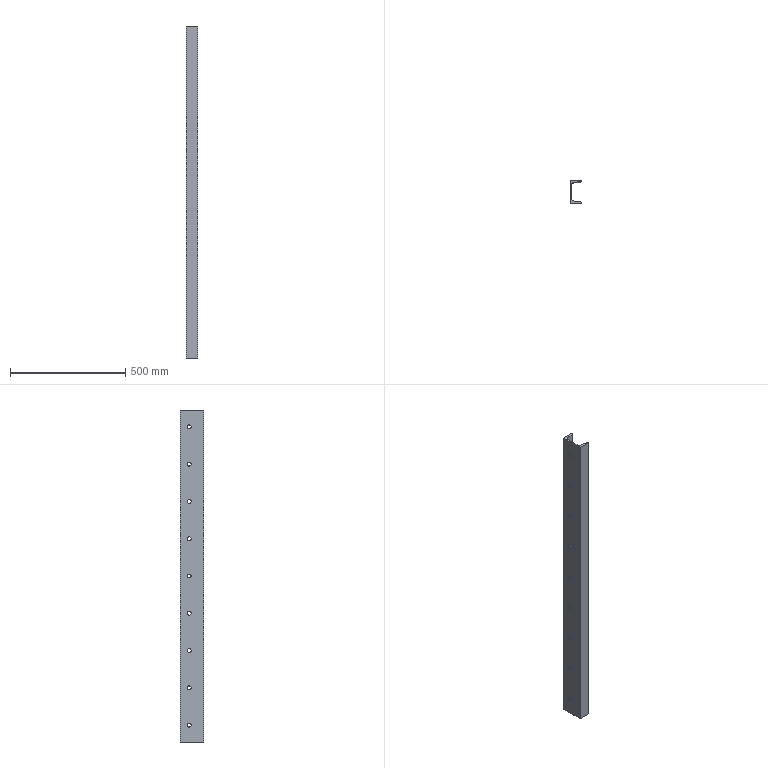Part | SolidWorks | features Extrusion 1, ICE 1 | 1 solid | 32 faces | box 50 x 100 x 1440 mm | volume 1898453 mm3 | cylinder 22 | plane 10 | commonest cylinder face diameters 17 x20 9 x2
STEP:
#1=CARTESIAN_POINT('',(-44.,-29.5,73.2));
#2=VERTEX_POINT('',#1);
#3=CARTESIAN_POINT('',(-44.,-46.5,73.2));
#4=VERTEX_POINT('',#3);
#5=CARTESIAN_POINT('',(-44.,-38.,73.2));
#6=DIRECTION('',(-1.,0.,0.));
#7=DIRECTION('',(0.,0.,1.));
#8=AXIS2_PLACEMENT_3D('',#5,#6,#7);
#9=CIRCLE('',#8,8.5);
#10=EDGE_CURVE('',#2,#4,#9,.T.);
#11=ORIENTED_EDGE('',*,*,#10,.F.);
#12=CARTESIAN_POINT('',(-50.,-29.5,73.2));
#13=VERTEX_POINT('',#12);
#14=CARTESIAN_POINT('',(1390.,-29.5,73.2));
#15=DIRECTION('',(-1.,0.,0.));
#16=VECTOR('',#15,1000.);
#17=LINE('',#14,#16);
#18=EDGE_CURVE('',#2,#13,#17,.T.);
#19=ORIENTED_EDGE('',*,*,#18,.T.);
#20=CARTESIAN_POINT('',(-50.,-46.5,73.2));
#21=VERTEX_POINT('',#20);
#22=CARTESIAN_POINT('',(-50.,-38.,73.2));
#23=DIRECTION('',(-1.,0.,0.));
#24=DIRECTION('',(0.,-1.,0.));
#25=AXIS2_PLACEMENT_3D('',#22,#23,#24);
#26=CIRCLE('',#25,8.5);
#27=EDGE_CURVE('',#13,#21,#26,.T.);
#28=ORIENTED_EDGE('',*,*,#27,.T.);
#29=CARTESIAN_POINT('',(1390.,-46.5,73.2));
#30=DIRECTION('',(-1.,0.,0.));
#31=VECTOR('',#30,1000.);
#32=LINE('',#29,#31);
#33=EDGE_CURVE('',#4,#21,#32,.T.);
#34=ORIENTED_EDGE('',*,*,#33,.F.);
#35=EDGE_LOOP('',(#11,#19,#28,#34));
#36=FACE_OUTER_BOUND('',#35,.T.);
#37=CARTESIAN_POINT('',(1390.,-38.,73.2));
#38=DIRECTION('',(-1.,0.,0.));
#39=DIRECTION('',(0.,-1.,0.));
#40=AXIS2_PLACEMENT_3D('',#37,#38,#39);
#41=CYLINDRICAL_SURFACE('',#40,8.5);
#42=ADVANCED_FACE('',(#36),#41,.F.);
#43=CARTESIAN_POINT('',(-44.,-29.5,234.9));
#44=VERTEX_POINT('',#43);
#45=CARTESIAN_POINT('',(-44.,-46.5,234.9));
#46=VERTEX_POINT('',#45);
#47=CARTESIAN_POINT('',(-44.,-38.,234.9));
#48=DIRECTION('',(-1.,0.,0.));
#49=DIRECTION('',(0.,0.,1.));
#50=AXIS2_PLACEMENT_3D('',#47,#48,#49);
#51=CIRCLE('',#50,8.5);
#52=EDGE_CURVE('',#44,#46,#51,.T.);
#53=ORIENTED_EDGE('',*,*,#52,.F.);
#54=CARTESIAN_POINT('',(-50.,-29.5,234.9));
#55=VERTEX_POINT('',#54);
#56=CARTESIAN_POINT('',(1390.,-29.5,234.9));
#57=DIRECTION('',(-1.,0.,0.));
#58=VECTOR('',#57,1000.);
#59=LINE('',#56,#58);
#60=EDGE_CURVE('',#44,#55,#59,.T.);
#61=ORIENTED_EDGE('',*,*,#60,.T.);
#62=CARTESIAN_POINT('',(-50.,-46.5,234.9));
#63=VERTEX_POINT('',#62);
#64=CARTESIAN_POINT('',(-50.,-38.,234.9));
#65=DIRECTION('',(-1.,0.,0.));
#66=DIRECTION('',(0.,-1.,0.));
#67=AXIS2_PLACEMENT_3D('',#64,#65,#66);
#68=CIRCLE('',#67,8.5);
#69=EDGE_CURVE('',#55,#63,#68,.T.);
#70=ORIENTED_EDGE('',*,*,#69,.T.);
#71=CARTESIAN_POINT('',(1390.,-46.5,234.9));
#72=DIRECTION('',(-1.,0.,0.));
#73=VECTOR('',#72,1000.);
#74=LINE('',#71,#73);
#75=EDGE_CURVE('',#46,#63,#74,.T.);
#76=ORIENTED_EDGE('',*,*,#75,.F.);
#77=EDGE_LOOP('',(#53,#61,#70,#76));
#78=FACE_OUTER_BOUND('',#77,.T.);
#79=CARTESIAN_POINT('',(1390.,-38.,234.9));
#80=DIRECTION('',(-1.,0.,0.));
#81=DIRECTION('',(0.,-1.,0.));
#82=AXIS2_PLACEMENT_3D('',#79,#80,#81);
#83=CYLINDRICAL_SURFACE('',#82,8.5);
#84=ADVANCED_FACE('',(#78),#83,.F.);
#85=CARTESIAN_POINT('',(-44.,-29.5,396.6));
#86=VERTEX_POINT('',#85);
#87=CARTESIAN_POINT('',(-44.,-46.5,396.6));
#88=VERTEX_POINT('',#87);
#89=CARTESIAN_POINT('',(-44.,-38.,396.6));
#90=DIRECTION('',(-1.,0.,0.));
#91=DIRECTION('',(0.,0.,1.));
#92=AXIS2_PLACEMENT_3D('',#89,#90,#91);
#93=CIRCLE('',#92,8.5);
#94=EDGE_CURVE('',#86,#88,#93,.T.);
#95=ORIENTED_EDGE('',*,*,#94,.F.);
#96=CARTESIAN_POINT('',(-50.,-29.5,396.6));
#97=VERTEX_POINT('',#96);
#98=CARTESIAN_POINT('',(1390.,-29.5,396.6));
#99=DIRECTION('',(-1.,0.,0.));
#100=VECTOR('',#99,1000.);
#101=LINE('',#98,#100);
#102=EDGE_CURVE('',#86,#97,#101,.T.);
#103=ORIENTED_EDGE('',*,*,#102,.T.);
#104=CARTESIAN_POINT('',(-50.,-46.5,396.6));
#105=VERTEX_POINT('',#104);
#106=CARTESIAN_POINT('',(-50.,-38.,396.6));
#107=DIRECTION('',(-1.,0.,0.));
#108=DIRECTION('',(0.,-1.,0.));
#109=AXIS2_PLACEMENT_3D('',#106,#107,#108);
#110=CIRCLE('',#109,8.5);
#111=EDGE_CURVE('',#97,#105,#110,.T.);
#112=ORIENTED_EDGE('',*,*,#111,.T.);
#113=CARTESIAN_POINT('',(1390.,-46.5,396.6));
#114=DIRECTION('',(-1.,0.,0.));
#115=VECTOR('',#114,1000.);
#116=LINE('',#113,#115);
#117=EDGE_CURVE('',#88,#105,#116,.T.);
#118=ORIENTED_EDGE('',*,*,#117,.F.);
#119=EDGE_LOOP('',(#95,#103,#112,#118));
#120=FACE_OUTER_BOUND('',#119,.T.);
#121=CARTESIAN_POINT('',(1390.,-38.,396.6));
#122=DIRECTION('',(-1.,0.,0.));
#123=DIRECTION('',(0.,-1.,0.));
#124=AXIS2_PLACEMENT_3D('',#121,#122,#123);
#125=CYLINDRICAL_SURFACE('',#124,8.5);
#126=ADVANCED_FACE('',(#120),#125,.F.);
#127=CARTESIAN_POINT('',(-44.,-29.5,558.3));
#128=VERTEX_POINT('',#127);
#129=CARTESIAN_POINT('',(-44.,-46.5,558.3));
#130=VERTEX_POINT('',#129);
#131=CARTESIAN_POINT('',(-44.,-38.,558.3));
#132=DIRECTION('',(-1.,0.,0.));
#133=DIRECTION('',(0.,0.,1.));
#134=AXIS2_PLACEMENT_3D('',#131,#132,#133);
#135=CIRCLE('',#134,8.5);
#136=EDGE_CURVE('',#128,#130,#135,.T.);
#137=ORIENTED_EDGE('',*,*,#136,.F.);
#138=CARTESIAN_POINT('',(-50.,-29.5,558.3));
#139=VERTEX_POINT('',#138);
#140=CARTESIAN_POINT('',(1390.,-29.5,558.3));
#141=DIRECTION('',(-1.,0.,0.));
#142=VECTOR('',#141,1000.);
#143=LINE('',#140,#142);
#144=EDGE_CURVE('',#128,#139,#143,.T.);
#145=ORIENTED_EDGE('',*,*,#144,.T.);
#146=CARTESIAN_POINT('',(-50.,-46.5,558.3));
#147=VERTEX_POINT('',#146);
#148=CARTESIAN_POINT('',(-50.,-38.,558.3));
#149=DIRECTION('',(-1.,0.,0.));
#150=DIRECTION('',(0.,-1.,0.));
#151=AXIS2_PLACEMENT_3D('',#148,#149,#150);
#152=CIRCLE('',#151,8.5);
#153=EDGE_CURVE('',#139,#147,#152,.T.);
#154=ORIENTED_EDGE('',*,*,#153,.T.);
#155=CARTESIAN_POINT('',(1390.,-46.5,558.3));
#156=DIRECTION('',(-1.,0.,0.));
#157=VECTOR('',#156,1000.);
#158=LINE('',#155,#157);
#159=EDGE_CURVE('',#130,#147,#158,.T.);
#160=ORIENTED_EDGE('',*,*,#159,.F.);
#161=EDGE_LOOP('',(#137,#145,#154,#160));
#162=FACE_OUTER_BOUND('',#161,.T.);
#163=CARTESIAN_POINT('',(1390.,-38.,558.3));
#164=DIRECTION('',(-1.,0.,0.));
#165=DIRECTION('',(0.,-1.,0.));
#166=AXIS2_PLACEMENT_3D('',#163,#164,#165);
#167=CYLINDRICAL_SURFACE('',#166,8.5);
#168=ADVANCED_FACE('',(#162),#167,.F.);
#169=CARTESIAN_POINT('',(-44.,-29.5,720.));
#170=VERTEX_POINT('',#169);
#171=CARTESIAN_POINT('',(-44.,-46.5,720.));
#172=VERTEX_POINT('',#171);
#173=CARTESIAN_POINT('',(-44.,-38.,720.));
#174=DIRECTION('',(-1.,0.,0.));
#175=DIRECTION('',(0.,0.,1.));
#176=AXIS2_PLACEMENT_3D('',#173,#174,#175);
#177=CIRCLE('',#176,8.5);
#178=EDGE_CURVE('',#170,#172,#177,.T.);
#179=ORIENTED_EDGE('',*,*,#178,.F.);
#180=CARTESIAN_POINT('',(-50.,-29.5,720.));
#181=VERTEX_POINT('',#180);
#182=CARTESIAN_POINT('',(1390.,-29.5,720.));
#183=DIRECTION('',(-1.,0.,0.));
#184=VECTOR('',#183,1000.);
#185=LINE('',#182,#184);
#186=EDGE_CURVE('',#170,#181,#185,.T.);
#187=ORIENTED_EDGE('',*,*,#186,.T.);
#188=CARTESIAN_POINT('',(-50.,-46.5,720.));
#189=VERTEX_POINT('',#188);
#190=CARTESIAN_POINT('',(-50.,-38.,720.));
#191=DIRECTION('',(-1.,0.,0.));
#192=DIRECTION('',(0.,-1.,0.));
#193=AXIS2_PLACEMENT_3D('',#190,#191,#192);
#194=CIRCLE('',#193,8.5);
#195=EDGE_CURVE('',#181,#189,#194,.T.);
#196=ORIENTED_EDGE('',*,*,#195,.T.);
#197=CARTESIAN_POINT('',(1390.,-46.5,720.));
#198=DIRECTION('',(-1.,0.,0.));
#199=VECTOR('',#198,1000.);
#200=LINE('',#197,#199);
#201=EDGE_CURVE('',#172,#189,#200,.T.);
#202=ORIENTED_EDGE('',*,*,#201,.F.);
#203=EDGE_LOOP('',(#179,#187,#196,#202));
#204=FACE_OUTER_BOUND('',#203,.T.);
#205=CARTESIAN_POINT('',(1390.,-38.,720.));
#206=DIRECTION('',(-1.,0.,0.));
#207=DIRECTION('',(0.,-1.,0.));
#208=AXIS2_PLACEMENT_3D('',#205,#206,#207);
#209=CYLINDRICAL_SURFACE('',#208,8.5);
#210=ADVANCED_FACE('',(#204),#209,.F.);
#211=CARTESIAN_POINT('',(-44.,-29.5,881.7));
#212=VERTEX_POINT('',#211);
#213=CARTESIAN_POINT('',(-44.,-46.5,881.7));
#214=VERTEX_POINT('',#213);
#215=CARTESIAN_POINT('',(-44.,-38.,881.7));
#216=DIRECTION('',(-1.,0.,0.));
#217=DIRECTION('',(0.,0.,1.));
#218=AXIS2_PLACEMENT_3D('',#215,#216,#217);
#219=CIRCLE('',#218,8.5);
#220=EDGE_CURVE('',#212,#214,#219,.T.);
#221=ORIENTED_EDGE('',*,*,#220,.F.);
#222=CARTESIAN_POINT('',(-50.,-29.5,881.7));
#223=VERTEX_POINT('',#222);
#224=CARTESIAN_POINT('',(1390.,-29.5,881.7));
#225=DIRECTION('',(-1.,0.,0.));
#226=VECTOR('',#225,1000.);
#227=LINE('',#224,#226);
#228=EDGE_CURVE('',#212,#223,#227,.T.);
#229=ORIENTED_EDGE('',*,*,#228,.T.);
#230=CARTESIAN_POINT('',(-50.,-46.5,881.7));
#231=VERTEX_POINT('',#230);
#232=CARTESIAN_POINT('',(-50.,-38.,881.7));
#233=DIRECTION('',(-1.,0.,0.));
#234=DIRECTION('',(0.,-1.,0.));
#235=AXIS2_PLACEMENT_3D('',#232,#233,#234);
#236=CIRCLE('',#235,8.5);
#237=EDGE_CURVE('',#223,#231,#236,.T.);
#238=ORIENTED_EDGE('',*,*,#237,.T.);
#239=CARTESIAN_POINT('',(1390.,-46.5,881.7));
#240=DIRECTION('',(-1.,0.,0.));
#241=VECTOR('',#240,1000.);
#242=LINE('',#239,#241);
#243=EDGE_CURVE('',#214,#231,#242,.T.);
#244=ORIENTED_EDGE('',*,*,#243,.F.);
#245=EDGE_LOOP('',(#221,#229,#238,#244));
#246=FACE_OUTER_BOUND('',#245,.T.);
#247=CARTESIAN_POINT('',(1390.,-38.,881.7));
#248=DIRECTION('',(-1.,0.,0.));
#249=DIRECTION('',(0.,-1.,0.));
#250=AXIS2_PLACEMENT_3D('',#247,#248,#249);
#251=CYLINDRICAL_SURFACE('',#250,8.5);
#252=ADVANCED_FACE('',(#246),#251,.F.);
#253=CARTESIAN_POINT('',(-44.,-29.5,1043.4));
#254=VERTEX_POINT('',#253);
#255=CARTESIAN_POINT('',(-44.,-46.5,1043.4));
#256=VERTEX_POINT('',#255);
#257=CARTESIAN_POINT('',(-44.,-38.,1043.4));
#258=DIRECTION('',(-1.,0.,0.));
#259=DIRECTION('',(0.,0.,1.));
#260=AXIS2_PLACEMENT_3D('',#257,#258,#259);
#261=CIRCLE('',#260,8.5);
#262=EDGE_CURVE('',#254,#256,#261,.T.);
#263=ORIENTED_EDGE('',*,*,#262,.F.);
#264=CARTESIAN_POINT('',(-50.,-29.5,1043.4));
#265=VERTEX_POINT('',#264);
#266=CARTESIAN_POINT('',(1390.,-29.5,1043.4));
#267=DIRECTION('',(-1.,0.,0.));
#268=VECTOR('',#267,1000.);
#269=LINE('',#266,#268);
#270=EDGE_CURVE('',#254,#265,#269,.T.);
#271=ORIENTED_EDGE('',*,*,#270,.T.);
#272=CARTESIAN_POINT('',(-50.,-46.5,1043.4));
#273=VERTEX_POINT('',#272);
#274=CARTESIAN_POINT('',(-50.,-38.,1043.4));
#275=DIRECTION('',(-1.,0.,0.));
#276=DIRECTION('',(0.,-1.,0.));
#277=AXIS2_PLACEMENT_3D('',#274,#275,#276);
#278=CIRCLE('',#277,8.5);
#279=EDGE_CURVE('',#265,#273,#278,.T.);
#280=ORIENTED_EDGE('',*,*,#279,.T.);
#281=CARTESIAN_POINT('',(1390.,-46.5,1043.4));
#282=DIRECTION('',(-1.,0.,0.));
#283=VECTOR('',#282,1000.);
#284=LINE('',#281,#283);
#285=EDGE_CURVE('',#256,#273,#284,.T.);
#286=ORIENTED_EDGE('',*,*,#285,.F.);
#287=EDGE_LOOP('',(#263,#271,#280,#286));
#288=FACE_OUTER_BOUND('',#287,.T.);
#289=CARTESIAN_POINT('',(1390.,-38.,1043.4));
#290=DIRECTION('',(-1.,0.,0.));
#291=DIRECTION('',(0.,-1.,0.));
#292=AXIS2_PLACEMENT_3D('',#289,#290,#291);
#293=CYLINDRICAL_SURFACE('',#292,8.5);
#294=ADVANCED_FACE('',(#288),#293,.F.);
#295=CARTESIAN_POINT('',(-44.,-29.5,1205.1));
#296=VERTEX_POINT('',#295);
#297=CARTESIAN_POINT('',(-44.,-46.5,1205.1));
#298=VERTEX_POINT('',#297);
#299=CARTESIAN_POINT('',(-44.,-38.,1205.1));
#300=DIRECTION('',(-1.,0.,0.));
#301=DIRECTION('',(0.,0.,1.));
#302=AXIS2_PLACEMENT_3D('',#299,#300,#301);
#303=CIRCLE('',#302,8.5);
#304=EDGE_CURVE('',#296,#298,#303,.T.);
#305=ORIENTED_EDGE('',*,*,#304,.F.);
#306=CARTESIAN_POINT('',(-50.,-29.5,1205.1));
#307=VERTEX_POINT('',#306);
#308=CARTESIAN_POINT('',(1390.,-29.5,1205.1));
#309=DIRECTION('',(-1.,0.,0.));
#310=VECTOR('',#309,1000.);
#311=LINE('',#308,#310);
#312=EDGE_CURVE('',#296,#307,#311,.T.);
#313=ORIENTED_EDGE('',*,*,#312,.T.);
#314=CARTESIAN_POINT('',(-50.,-46.5,1205.1));
#315=VERTEX_POINT('',#314);
#316=CARTESIAN_POINT('',(-50.,-38.,1205.1));
#317=DIRECTION('',(-1.,0.,0.));
#318=DIRECTION('',(0.,-1.,0.));
#319=AXIS2_PLACEMENT_3D('',#316,#317,#318);
#320=CIRCLE('',#319,8.5);
#321=EDGE_CURVE('',#307,#315,#320,.T.);
#322=ORIENTED_EDGE('',*,*,#321,.T.);
#323=CARTESIAN_POINT('',(1390.,-46.5,1205.1));
#324=DIRECTION('',(-1.,0.,0.));
#325=VECTOR('',#324,1000.);
#326=LINE('',#323,#325);
#327=EDGE_CURVE('',#298,#315,#326,.T.);
#328=ORIENTED_EDGE('',*,*,#327,.F.);
#329=EDGE_LOOP('',(#305,#313,#322,#328));
#330=FACE_OUTER_BOUND('',#329,.T.);
#331=CARTESIAN_POINT('',(1390.,-38.,1205.1));
#332=DIRECTION('',(-1.,0.,0.));
#333=DIRECTION('',(0.,-1.,0.));
#334=AXIS2_PLACEMENT_3D('',#331,#332,#333);
#335=CYLINDRICAL_SURFACE('',#334,8.5);
#336=ADVANCED_FACE('',(#330),#335,.F.);
#337=CARTESIAN_POINT('',(-44.,-29.5,1366.8));
#338=VERTEX_POINT('',#337);
#339=CARTESIAN_POINT('',(-44.,-46.5,1366.8));
#340=VERTEX_POINT('',#339);
#341=CARTESIAN_POINT('',(-44.,-38.,1366.8));
#342=DIRECTION('',(-1.,0.,0.));
#343=DIRECTION('',(0.,0.,1.));
#344=AXIS2_PLACEMENT_3D('',#341,#342,#343);
#345=CIRCLE('',#344,8.5);
#346=EDGE_CURVE('',#338,#340,#345,.T.);
#347=ORIENTED_EDGE('',*,*,#346,.F.);
#348=CARTESIAN_POINT('',(-50.,-29.5,1366.8));
#349=VERTEX_POINT('',#348);
#350=CARTESIAN_POINT('',(1390.,-29.5,1366.8));
#351=DIRECTION('',(-1.,0.,0.));
#352=VECTOR('',#351,1000.);
#353=LINE('',#350,#352);
#354=EDGE_CURVE('',#338,#349,#353,.T.);
#355=ORIENTED_EDGE('',*,*,#354,.T.);
#356=CARTESIAN_POINT('',(-50.,-46.5,1366.8));
#357=VERTEX_POINT('',#356);
#358=CARTESIAN_POINT('',(-50.,-38.,1366.8));
#359=DIRECTION('',(-1.,0.,0.));
#360=DIRECTION('',(0.,-1.,0.));
#361=AXIS2_PLACEMENT_3D('',#358,#359,#360);
#362=CIRCLE('',#361,8.5);
#363=EDGE_CURVE('',#349,#357,#362,.T.);
#364=ORIENTED_EDGE('',*,*,#363,.T.);
#365=CARTESIAN_POINT('',(1390.,-46.5,1366.8));
#366=DIRECTION('',(-1.,0.,0.));
#367=VECTOR('',#366,1000.);
#368=LINE('',#365,#367);
#369=EDGE_CURVE('',#340,#357,#368,.T.);
#370=ORIENTED_EDGE('',*,*,#369,.F.);
#371=EDGE_LOOP('',(#347,#355,#364,#370));
#372=FACE_OUTER_BOUND('',#371,.T.);
#373=CARTESIAN_POINT('',(1390.,-38.,1366.8));
#374=DIRECTION('',(-1.,0.,0.));
#375=DIRECTION('',(0.,-1.,0.));
#376=AXIS2_PLACEMENT_3D('',#373,#374,#375);
#377=CYLINDRICAL_SURFACE('',#376,8.5);
#378=ADVANCED_FACE('',(#372),#377,.F.);
#379=CARTESIAN_POINT('',(0.,-1.075,0.));
#380=VERTEX_POINT('',#379);
#381=CARTESIAN_POINT('',(0.,0.,0.));
#382=VERTEX_POINT('',#381);
#383=CARTESIAN_POINT('',(0.,-1.075,0.));
#384=DIRECTION('',(0.,1.,0.));
#385=VECTOR('',#384,1000.);
#386=LINE('',#383,#385);
#387=EDGE_CURVE('',#380,#382,#386,.T.);
#388=ORIENTED_EDGE('',*,*,#387,.T.);
#389=CARTESIAN_POINT('',(0.,0.,1440.));
#390=VERTEX_POINT('',#389);
#391=CARTESIAN_POINT('',(0.,0.,1440.));
#392=DIRECTION('',(0.,0.,-1.));
#393=VECTOR('',#392,1000.);
#394=LINE('',#391,#393);
#395=EDGE_CURVE('',#390,#382,#394,.T.);
#396=ORIENTED_EDGE('',*,*,#395,.F.);
#397=CARTESIAN_POINT('',(0.,-1.075,1440.));
#398=VERTEX_POINT('',#397);
#399=CARTESIAN_POINT('',(0.,-1.075,1440.));
#400=DIRECTION('',(0.,1.,0.));
#401=VECTOR('',#400,1000.);
#402=LINE('',#399,#401);
#403=EDGE_CURVE('',#398,#390,#402,.T.);
#404=ORIENTED_EDGE('',*,*,#403,.F.);
#405=CARTESIAN_POINT('',(0.,-1.075,1440.));
#406=DIRECTION('',(0.,0.,-1.));
#407=VECTOR('',#406,1000.);
#408=LINE('',#405,#407);
#409=EDGE_CURVE('',#398,#380,#408,.T.);
#410=ORIENTED_EDGE('',*,*,#409,.T.);
#411=EDGE_LOOP('',(#388,#396,#404,#410));
#412=FACE_OUTER_BOUND('',#411,.T.);
#413=CARTESIAN_POINT('',(0.,-1.075,1440.));
#414=DIRECTION('',(-1.,0.,0.));
#415=DIRECTION('',(0.,0.,1.));
#416=AXIS2_PLACEMENT_3D('',#413,#414,#415);
#417=PLANE('',#416);
#418=ADVANCED_FACE('',(#412),#417,.F.);
#419=CARTESIAN_POINT('',(-50.,0.,0.));
#420=VERTEX_POINT('',#419);
#421=CARTESIAN_POINT('',(0.,0.,0.));
#422=DIRECTION('',(-1.,0.,0.));
#423=VECTOR('',#422,1000.);
#424=LINE('',#421,#423);
#425=EDGE_CURVE('',#382,#420,#424,.T.);
#426=ORIENTED_EDGE('',*,*,#425,.T.);
#427=CARTESIAN_POINT('',(-50.,0.,1440.));
#428=VERTEX_POINT('',#427);
#429=CARTESIAN_POINT('',(-50.,0.,1440.));
#430=DIRECTION('',(0.,0.,-1.));
#431=VECTOR('',#430,1000.);
#432=LINE('',#429,#431);
#433=EDGE_CURVE('',#428,#420,#432,.T.);
#434=ORIENTED_EDGE('',*,*,#433,.F.);
#435=CARTESIAN_POINT('',(0.,0.,1440.));
#436=DIRECTION('',(-1.,0.,0.));
#437=VECTOR('',#436,1000.);
#438=LINE('',#435,#437);
#439=EDGE_CURVE('',#390,#428,#438,.T.);
#440=ORIENTED_EDGE('',*,*,#439,.F.);
#441=ORIENTED_EDGE('',*,*,#395,.T.);
#442=EDGE_LOOP('',(#426,#434,#440,#441));
#443=FACE_OUTER_BOUND('',#442,.T.);
#444=CARTESIAN_POINT('',(0.,0.,1440.));
#445=DIRECTION('',(0.,-1.,0.));
#446=DIRECTION('',(1.,0.,0.));
#447=AXIS2_PLACEMENT_3D('',#444,#445,#446);
#448=PLANE('',#447);
#449=ADVANCED_FACE('',(#443),#448,.F.);
#450=CARTESIAN_POINT('',(-50.,-38.,73.2));
#451=DIRECTION('',(-1.,0.,0.));
#452=DIRECTION('',(0.,-1.,0.));
#453=AXIS2_PLACEMENT_3D('',#450,#451,#452);
#454=CIRCLE('',#453,8.5);
#455=EDGE_CURVE('',#21,#13,#454,.T.);
#456=ORIENTED_EDGE('',*,*,#455,.F.);
#457=ORIENTED_EDGE('',*,*,#27,.F.);
#458=EDGE_LOOP('',(#456,#457));
#459=FACE_BOUND('',#458,.T.);
#460=CARTESIAN_POINT('',(-50.,-38.,234.9));
#461=DIRECTION('',(-1.,0.,0.));
#462=DIRECTION('',(0.,-1.,0.));
#463=AXIS2_PLACEMENT_3D('',#460,#461,#462);
#464=CIRCLE('',#463,8.5);
#465=EDGE_CURVE('',#63,#55,#464,.T.);
#466=ORIENTED_EDGE('',*,*,#465,.F.);
#467=ORIENTED_EDGE('',*,*,#69,.F.);
#468=EDGE_LOOP('',(#466,#467));
#469=FACE_BOUND('',#468,.T.);
#470=CARTESIAN_POINT('',(-50.,-38.,396.6));
#471=DIRECTION('',(-1.,0.,0.));
#472=DIRECTION('',(0.,-1.,0.));
#473=AXIS2_PLACEMENT_3D('',#470,#471,#472);
#474=CIRCLE('',#473,8.5);
#475=EDGE_CURVE('',#105,#97,#474,.T.);
#476=ORIENTED_EDGE('',*,*,#475,.F.);
#477=ORIENTED_EDGE('',*,*,#111,.F.);
#478=EDGE_LOOP('',(#476,#477));
#479=FACE_BOUND('',#478,.T.);
#480=CARTESIAN_POINT('',(-50.,-38.,558.3));
#481=DIRECTION('',(-1.,0.,0.));
#482=DIRECTION('',(0.,-1.,0.));
#483=AXIS2_PLACEMENT_3D('',#480,#481,#482);
#484=CIRCLE('',#483,8.5);
#485=EDGE_CURVE('',#147,#139,#484,.T.);
#486=ORIENTED_EDGE('',*,*,#485,.F.);
#487=ORIENTED_EDGE('',*,*,#153,.F.);
#488=EDGE_LOOP('',(#486,#487));
#489=FACE_BOUND('',#488,.T.);
#490=CARTESIAN_POINT('',(-50.,-38.,720.));
#491=DIRECTION('',(-1.,0.,0.));
#492=DIRECTION('',(0.,-1.,0.));
#493=AXIS2_PLACEMENT_3D('',#490,#491,#492);
#494=CIRCLE('',#493,8.5);
#495=EDGE_CURVE('',#189,#181,#494,.T.);
#496=ORIENTED_EDGE('',*,*,#495,.F.);
#497=ORIENTED_EDGE('',*,*,#195,.F.);
#498=EDGE_LOOP('',(#496,#497));
#499=FACE_BOUND('',#498,.T.);
#500=CARTESIAN_POINT('',(-50.,-38.,881.7));
#501=DIRECTION('',(-1.,0.,0.));
#502=DIRECTION('',(0.,-1.,0.));
#503=AXIS2_PLACEMENT_3D('',#500,#501,#502);
#504=CIRCLE('',#503,8.5);
#505=EDGE_CURVE('',#231,#223,#504,.T.);
#506=ORIENTED_EDGE('',*,*,#505,.F.);
#507=ORIENTED_EDGE('',*,*,#237,.F.);
#508=EDGE_LOOP('',(#506,#507));
#509=FACE_BOUND('',#508,.T.);
#510=CARTESIAN_POINT('',(-50.,-38.,1043.4));
#511=DIRECTION('',(-1.,0.,0.));
#512=DIRECTION('',(0.,-1.,0.));
#513=AXIS2_PLACEMENT_3D('',#510,#511,#512);
#514=CIRCLE('',#513,8.5);
#515=EDGE_CURVE('',#273,#265,#514,.T.);
#516=ORIENTED_EDGE('',*,*,#515,.F.);
#517=ORIENTED_EDGE('',*,*,#279,.F.);
#518=EDGE_LOOP('',(#516,#517));
#519=FACE_BOUND('',#518,.T.);
#520=CARTESIAN_POINT('',(-50.,-38.,1205.1));
#521=DIRECTION('',(-1.,0.,0.));
#522=DIRECTION('',(0.,-1.,0.));
#523=AXIS2_PLACEMENT_3D('',#520,#521,#522);
#524=CIRCLE('',#523,8.5);
#525=EDGE_CURVE('',#315,#307,#524,.T.);
#526=ORIENTED_EDGE('',*,*,#525,.F.);
#527=ORIENTED_EDGE('',*,*,#321,.F.);
#528=EDGE_LOOP('',(#526,#527));
#529=FACE_BOUND('',#528,.T.);
#530=CARTESIAN_POINT('',(-50.,-38.,1366.8));
#531=DIRECTION('',(-1.,0.,0.));
#532=DIRECTION('',(0.,-1.,0.));
#533=AXIS2_PLACEMENT_3D('',#530,#531,#532);
#534=CIRCLE('',#533,8.5);
#535=EDGE_CURVE('',#357,#349,#534,.T.);
#536=ORIENTED_EDGE('',*,*,#535,.F.);
#537=ORIENTED_EDGE('',*,*,#363,.F.);
#538=EDGE_LOOP('',(#536,#537));
#539=FACE_BOUND('',#538,.T.);
#540=CARTESIAN_POINT('',(-50.,-100.,0.));
#541=VERTEX_POINT('',#540);
#542=CARTESIAN_POINT('',(-50.,0.,0.));
#543=DIRECTION('',(0.,-1.,0.));
#544=VECTOR('',#543,1000.);
#545=LINE('',#542,#544);
#546=EDGE_CURVE('',#420,#541,#545,.T.);
#547=ORIENTED_EDGE('',*,*,#546,.T.);
#548=CARTESIAN_POINT('',(-50.,-100.,1440.));
#549=VERTEX_POINT('',#548);
#550=CARTESIAN_POINT('',(-50.,-100.,1440.));
#551=DIRECTION('',(0.,0.,-1.));
#552=VECTOR('',#551,1000.);
#553=LINE('',#550,#552);
#554=EDGE_CURVE('',#549,#541,#553,.T.);
#555=ORIENTED_EDGE('',*,*,#554,.F.);
#556=CARTESIAN_POINT('',(-50.,0.,1440.));
#557=DIRECTION('',(0.,-1.,0.));
#558=VECTOR('',#557,1000.);
#559=LINE('',#556,#558);
#560=EDGE_CURVE('',#428,#549,#559,.T.);
#561=ORIENTED_EDGE('',*,*,#560,.F.);
#562=ORIENTED_EDGE('',*,*,#433,.T.);
#563=EDGE_LOOP('',(#547,#555,#561,#562));
#564=FACE_OUTER_BOUND('',#563,.T.);
#565=CARTESIAN_POINT('',(-50.,0.,1440.));
#566=DIRECTION('',(1.,0.,0.));
#567=DIRECTION('',(0.,1.,0.));
#568=AXIS2_PLACEMENT_3D('',#565,#566,#567);
#569=PLANE('',#568);
#570=ADVANCED_FACE('',(#459,#469,#479,#489,#499,#509,#519,#529,#539,#564),#569,.F.);
#571=CARTESIAN_POINT('',(0.,-100.,0.));
#572=VERTEX_POINT('',#571);
#573=CARTESIAN_POINT('',(-50.,-100.,0.));
#574=DIRECTION('',(1.,0.,0.));
#575=VECTOR('',#574,1000.);
#576=LINE('',#573,#575);
#577=EDGE_CURVE('',#541,#572,#576,.T.);
#578=ORIENTED_EDGE('',*,*,#577,.T.);
#579=CARTESIAN_POINT('',(0.,-100.,1440.));
#580=VERTEX_POINT('',#579);
#581=CARTESIAN_POINT('',(0.,-100.,1440.));
#582=DIRECTION('',(0.,0.,-1.));
#583=VECTOR('',#582,1000.);
#584=LINE('',#581,#583);
#585=EDGE_CURVE('',#580,#572,#584,.T.);
#586=ORIENTED_EDGE('',*,*,#585,.F.);
#587=CARTESIAN_POINT('',(-50.,-100.,1440.));
#588=DIRECTION('',(1.,0.,0.));
#589=VECTOR('',#588,1000.);
#590=LINE('',#587,#589);
#591=EDGE_CURVE('',#549,#580,#590,.T.);
#592=ORIENTED_EDGE('',*,*,#591,.F.);
#593=ORIENTED_EDGE('',*,*,#554,.T.);
#594=EDGE_LOOP('',(#578,#586,#592,#593));
#595=FACE_OUTER_BOUND('',#594,.T.);
#596=CARTESIAN_POINT('',(-50.,-100.,1440.));
#597=DIRECTION('',(0.,1.,0.));
#598=DIRECTION('',(0.,0.,1.));
#599=AXIS2_PLACEMENT_3D('',#596,#597,#598);
#600=PLANE('',#599);
#601=ADVANCED_FACE('',(#595),#600,.F.);
#602=CARTESIAN_POINT('',(0.,-98.925,0.));
#603=VERTEX_POINT('',#602);
#604=CARTESIAN_POINT('',(0.,-100.,0.));
#605=DIRECTION('',(0.,1.,0.));
#606=VECTOR('',#605,1000.);
#607=LINE('',#604,#606);
#608=EDGE_CURVE('',#572,#603,#607,.T.);
#609=ORIENTED_EDGE('',*,*,#608,.T.);
#610=CARTESIAN_POINT('',(0.,-98.925,1440.));
#611=VERTEX_POINT('',#610);
#612=CARTESIAN_POINT('',(0.,-98.925,1440.));
#613=DIRECTION('',(0.,0.,-1.));
#614=VECTOR('',#613,1000.);
#615=LINE('',#612,#614);
#616=EDGE_CURVE('',#611,#603,#615,.T.);
#617=ORIENTED_EDGE('',*,*,#616,.F.);
#618=CARTESIAN_POINT('',(0.,-100.,1440.));
#619=DIRECTION('',(0.,1.,0.));
#620=VECTOR('',#619,1000.);
#621=LINE('',#618,#620);
#622=EDGE_CURVE('',#580,#611,#621,.T.);
#623=ORIENTED_EDGE('',*,*,#622,.F.);
#624=ORIENTED_EDGE('',*,*,#585,.T.);
#625=EDGE_LOOP('',(#609,#617,#623,#624));
#626=FACE_OUTER_BOUND('',#625,.T.);
#627=CARTESIAN_POINT('',(0.,-100.,1440.));
#628=DIRECTION('',(-1.,0.,0.));
#629=DIRECTION('',(0.,0.,1.));
#630=AXIS2_PLACEMENT_3D('',#627,#628,#629);
#631=PLANE('',#630);
#632=ADVANCED_FACE('',(#626),#631,.F.);
#633=CARTESIAN_POINT('',(-3.874,-94.469,0.));
#634=VERTEX_POINT('',#633);
#635=CARTESIAN_POINT('',(-4.5,-98.925,0.));
#636=DIRECTION('',(0.,0.,1.));
#637=DIRECTION('',(1.,0.,0.));
#638=AXIS2_PLACEMENT_3D('',#635,#636,#637);
#639=CIRCLE('',#638,4.5);
#640=EDGE_CURVE('',#603,#634,#639,.T.);
#641=ORIENTED_EDGE('',*,*,#640,.T.);
#642=CARTESIAN_POINT('',(-3.874,-94.469,1440.));
#643=VERTEX_POINT('',#642);
#644=CARTESIAN_POINT('',(-3.874,-94.469,1440.));
#645=DIRECTION('',(0.,0.,-1.));
#646=VECTOR('',#645,1000.);
#647=LINE('',#644,#646);
#648=EDGE_CURVE('',#643,#634,#647,.T.);
#649=ORIENTED_EDGE('',*,*,#648,.F.);
#650=CARTESIAN_POINT('',(-4.5,-98.925,1440.));
#651=DIRECTION('',(0.,0.,1.));
#652=DIRECTION('',(1.,0.,0.));
#653=AXIS2_PLACEMENT_3D('',#650,#651,#652);
#654=CIRCLE('',#653,4.5);
#655=EDGE_CURVE('',#611,#643,#654,.T.);
#656=ORIENTED_EDGE('',*,*,#655,.F.);
#657=ORIENTED_EDGE('',*,*,#616,.T.);
#658=EDGE_LOOP('',(#641,#649,#656,#657));
#659=FACE_OUTER_BOUND('',#658,.T.);
#660=CARTESIAN_POINT('',(-4.5,-98.925,1440.));
#661=DIRECTION('',(0.,0.,-1.));
#662=DIRECTION('',(-1.,0.,0.));
#663=AXIS2_PLACEMENT_3D('',#660,#661,#662);
#664=CYLINDRICAL_SURFACE('',#663,4.5);
#665=ADVANCED_FACE('',(#659),#664,.T.);
#666=CARTESIAN_POINT('',(-36.683,-89.858,0.));
#667=VERTEX_POINT('',#666);
#668=CARTESIAN_POINT('',(-3.874,-94.469,0.));
#669=DIRECTION('',(-0.9903,0.1392,0.));
#670=VECTOR('',#669,1000.);
#671=LINE('',#668,#670);
#672=EDGE_CURVE('',#634,#667,#671,.T.);
#673=ORIENTED_EDGE('',*,*,#672,.T.);
#674=CARTESIAN_POINT('',(-36.683,-89.858,1440.));
#675=VERTEX_POINT('',#674);
#676=CARTESIAN_POINT('',(-36.683,-89.858,1440.));
#677=DIRECTION('',(0.,0.,-1.));
#678=VECTOR('',#677,1000.);
#679=LINE('',#676,#678);
#680=EDGE_CURVE('',#675,#667,#679,.T.);
#681=ORIENTED_EDGE('',*,*,#680,.F.);
#682=CARTESIAN_POINT('',(-3.874,-94.469,1440.));
#683=DIRECTION('',(-0.9903,0.1392,0.));
#684=VECTOR('',#683,1000.);
#685=LINE('',#682,#684);
#686=EDGE_CURVE('',#643,#675,#685,.T.);
#687=ORIENTED_EDGE('',*,*,#686,.F.);
#688=ORIENTED_EDGE('',*,*,#648,.T.);
#689=EDGE_LOOP('',(#673,#681,#687,#688));
#690=FACE_OUTER_BOUND('',#689,.T.);
#691=CARTESIAN_POINT('',(-3.874,-94.469,1440.));
#692=DIRECTION('',(-0.1392,-0.9903,0.));
#693=DIRECTION('',(0.9903,-0.1392,0.));
#694=AXIS2_PLACEMENT_3D('',#691,#692,#693);
#695=PLANE('',#694);
#696=ADVANCED_FACE('',(#690),#695,.F.);
#697=CARTESIAN_POINT('',(-44.,-81.441,0.));
#698=VERTEX_POINT('',#697);
#699=CARTESIAN_POINT('',(-35.5,-81.441,0.));
#700=DIRECTION('',(0.,0.,-1.));
#701=DIRECTION('',(-1.,0.,0.));
#702=AXIS2_PLACEMENT_3D('',#699,#700,#701);
#703=CIRCLE('',#702,8.5);
#704=EDGE_CURVE('',#667,#698,#703,.T.);
#705=ORIENTED_EDGE('',*,*,#704,.T.);
#706=CARTESIAN_POINT('',(-44.,-81.441,1440.));
#707=VERTEX_POINT('',#706);
#708=CARTESIAN_POINT('',(-44.,-81.441,1440.));
#709=DIRECTION('',(0.,0.,-1.));
#710=VECTOR('',#709,1000.);
#711=LINE('',#708,#710);
#712=EDGE_CURVE('',#707,#698,#711,.T.);
#713=ORIENTED_EDGE('',*,*,#712,.F.);
#714=CARTESIAN_POINT('',(-35.5,-81.441,1440.));
#715=DIRECTION('',(0.,0.,-1.));
#716=DIRECTION('',(-1.,0.,0.));
#717=AXIS2_PLACEMENT_3D('',#714,#715,#716);
#718=CIRCLE('',#717,8.5);
#719=EDGE_CURVE('',#675,#707,#718,.T.);
#720=ORIENTED_EDGE('',*,*,#719,.F.);
#721=ORIENTED_EDGE('',*,*,#680,.T.);
#722=EDGE_LOOP('',(#705,#713,#720,#721));
#723=FACE_OUTER_BOUND('',#722,.T.);
#724=CARTESIAN_POINT('',(-35.5,-81.441,1440.));
#725=DIRECTION('',(0.,0.,-1.));
#726=DIRECTION('',(-1.,0.,0.));
#727=AXIS2_PLACEMENT_3D('',#724,#725,#726);
#728=CYLINDRICAL_SURFACE('',#727,8.5);
#729=ADVANCED_FACE('',(#723),#728,.F.);
#730=CARTESIAN_POINT('',(-44.,-38.,73.2));
#731=DIRECTION('',(-1.,0.,0.));
#732=DIRECTION('',(0.,0.,1.));
#733=AXIS2_PLACEMENT_3D('',#730,#731,#732);
#734=CIRCLE('',#733,8.5);
#735=EDGE_CURVE('',#4,#2,#734,.T.);
#736=ORIENTED_EDGE('',*,*,#735,.T.);
#737=ORIENTED_EDGE('',*,*,#10,.T.);
#738=EDGE_LOOP('',(#736,#737));
#739=FACE_BOUND('',#738,.T.);
#740=CARTESIAN_POINT('',(-44.,-38.,234.9));
#741=DIRECTION('',(-1.,0.,0.));
#742=DIRECTION('',(0.,0.,1.));
#743=AXIS2_PLACEMENT_3D('',#740,#741,#742);
#744=CIRCLE('',#743,8.5);
#745=EDGE_CURVE('',#46,#44,#744,.T.);
#746=ORIENTED_EDGE('',*,*,#745,.T.);
#747=ORIENTED_EDGE('',*,*,#52,.T.);
#748=EDGE_LOOP('',(#746,#747));
#749=FACE_BOUND('',#748,.T.);
#750=CARTESIAN_POINT('',(-44.,-38.,396.6));
#751=DIRECTION('',(-1.,0.,0.));
#752=DIRECTION('',(0.,0.,1.));
#753=AXIS2_PLACEMENT_3D('',#750,#751,#752);
#754=CIRCLE('',#753,8.5);
#755=EDGE_CURVE('',#88,#86,#754,.T.);
#756=ORIENTED_EDGE('',*,*,#755,.T.);
#757=ORIENTED_EDGE('',*,*,#94,.T.);
#758=EDGE_LOOP('',(#756,#757));
#759=FACE_BOUND('',#758,.T.);
#760=CARTESIAN_POINT('',(-44.,-38.,558.3));
#761=DIRECTION('',(-1.,0.,0.));
#762=DIRECTION('',(0.,0.,1.));
#763=AXIS2_PLACEMENT_3D('',#760,#761,#762);
#764=CIRCLE('',#763,8.5);
#765=EDGE_CURVE('',#130,#128,#764,.T.);
#766=ORIENTED_EDGE('',*,*,#765,.T.);
#767=ORIENTED_EDGE('',*,*,#136,.T.);
#768=EDGE_LOOP('',(#766,#767));
#769=FACE_BOUND('',#768,.T.);
#770=CARTESIAN_POINT('',(-44.,-38.,720.));
#771=DIRECTION('',(-1.,0.,0.));
#772=DIRECTION('',(0.,0.,1.));
#773=AXIS2_PLACEMENT_3D('',#770,#771,#772);
#774=CIRCLE('',#773,8.5);
#775=EDGE_CURVE('',#172,#170,#774,.T.);
#776=ORIENTED_EDGE('',*,*,#775,.T.);
#777=ORIENTED_EDGE('',*,*,#178,.T.);
#778=EDGE_LOOP('',(#776,#777));
#779=FACE_BOUND('',#778,.T.);
#780=CARTESIAN_POINT('',(-44.,-38.,881.7));
#781=DIRECTION('',(-1.,0.,0.));
#782=DIRECTION('',(0.,0.,1.));
#783=AXIS2_PLACEMENT_3D('',#780,#781,#782);
#784=CIRCLE('',#783,8.5);
#785=EDGE_CURVE('',#214,#212,#784,.T.);
#786=ORIENTED_EDGE('',*,*,#785,.T.);
#787=ORIENTED_EDGE('',*,*,#220,.T.);
#788=EDGE_LOOP('',(#786,#787));
#789=FACE_BOUND('',#788,.T.);
#790=CARTESIAN_POINT('',(-44.,-38.,1043.4));
#791=DIRECTION('',(-1.,0.,0.));
#792=DIRECTION('',(0.,0.,1.));
#793=AXIS2_PLACEMENT_3D('',#790,#791,#792);
#794=CIRCLE('',#793,8.5);
#795=EDGE_CURVE('',#256,#254,#794,.T.);
#796=ORIENTED_EDGE('',*,*,#795,.T.);
#797=ORIENTED_EDGE('',*,*,#262,.T.);
#798=EDGE_LOOP('',(#796,#797));
#799=FACE_BOUND('',#798,.T.);
#800=CARTESIAN_POINT('',(-44.,-38.,1205.1));
#801=DIRECTION('',(-1.,0.,0.));
#802=DIRECTION('',(0.,0.,1.));
#803=AXIS2_PLACEMENT_3D('',#800,#801,#802);
#804=CIRCLE('',#803,8.5);
#805=EDGE_CURVE('',#298,#296,#804,.T.);
#806=ORIENTED_EDGE('',*,*,#805,.T.);
#807=ORIENTED_EDGE('',*,*,#304,.T.);
#808=EDGE_LOOP('',(#806,#807));
#809=FACE_BOUND('',#808,.T.);
#810=CARTESIAN_POINT('',(-44.,-38.,1366.8));
#811=DIRECTION('',(-1.,0.,0.));
#812=DIRECTION('',(0.,0.,1.));
#813=AXIS2_PLACEMENT_3D('',#810,#811,#812);
#814=CIRCLE('',#813,8.5);
#815=EDGE_CURVE('',#340,#338,#814,.T.);
#816=ORIENTED_EDGE('',*,*,#815,.T.);
#817=ORIENTED_EDGE('',*,*,#346,.T.);
#818=EDGE_LOOP('',(#816,#817));
#819=FACE_BOUND('',#818,.T.);
#820=CARTESIAN_POINT('',(-44.,-18.559,0.));
#821=VERTEX_POINT('',#820);
#822=CARTESIAN_POINT('',(-44.,-81.441,0.));
#823=DIRECTION('',(0.,1.,0.));
#824=VECTOR('',#823,1000.);
#825=LINE('',#822,#824);
#826=EDGE_CURVE('',#698,#821,#825,.T.);
#827=ORIENTED_EDGE('',*,*,#826,.T.);
#828=CARTESIAN_POINT('',(-44.,-18.559,1440.));
#829=VERTEX_POINT('',#828);
#830=CARTESIAN_POINT('',(-44.,-18.559,1440.));
#831=DIRECTION('',(0.,0.,-1.));
#832=VECTOR('',#831,1000.);
#833=LINE('',#830,#832);
#834=EDGE_CURVE('',#829,#821,#833,.T.);
#835=ORIENTED_EDGE('',*,*,#834,.F.);
#836=CARTESIAN_POINT('',(-44.,-81.441,1440.));
#837=DIRECTION('',(0.,1.,0.));
#838=VECTOR('',#837,1000.);
#839=LINE('',#836,#838);
#840=EDGE_CURVE('',#707,#829,#839,.T.);
#841=ORIENTED_EDGE('',*,*,#840,.F.);
#842=ORIENTED_EDGE('',*,*,#712,.T.);
#843=EDGE_LOOP('',(#827,#835,#841,#842));
#844=FACE_OUTER_BOUND('',#843,.T.);
#845=CARTESIAN_POINT('',(-44.,-81.441,1440.));
#846=DIRECTION('',(-1.,0.,0.));
#847=DIRECTION('',(0.,0.,1.));
#848=AXIS2_PLACEMENT_3D('',#845,#846,#847);
#849=PLANE('',#848);
#850=ADVANCED_FACE('',(#739,#749,#759,#769,#779,#789,#799,#809,#819,#844),#849,.F.);
#851=CARTESIAN_POINT('',(-36.683,-10.142,0.));
#852=VERTEX_POINT('',#851);
#853=CARTESIAN_POINT('',(-35.5,-18.559,0.));
#854=DIRECTION('',(0.,0.,-1.));
#855=DIRECTION('',(-1.,0.,0.));
#856=AXIS2_PLACEMENT_3D('',#853,#854,#855);
#857=CIRCLE('',#856,8.5);
#858=EDGE_CURVE('',#821,#852,#857,.T.);
#859=ORIENTED_EDGE('',*,*,#858,.T.);
#860=CARTESIAN_POINT('',(-36.683,-10.142,1440.));
#861=VERTEX_POINT('',#860);
#862=CARTESIAN_POINT('',(-36.683,-10.142,1440.));
#863=DIRECTION('',(0.,0.,-1.));
#864=VECTOR('',#863,1000.);
#865=LINE('',#862,#864);
#866=EDGE_CURVE('',#861,#852,#865,.T.);
#867=ORIENTED_EDGE('',*,*,#866,.F.);
#868=CARTESIAN_POINT('',(-35.5,-18.559,1440.));
#869=DIRECTION('',(0.,0.,-1.));
#870=DIRECTION('',(-1.,0.,0.));
#871=AXIS2_PLACEMENT_3D('',#868,#869,#870);
#872=CIRCLE('',#871,8.5);
#873=EDGE_CURVE('',#829,#861,#872,.T.);
#874=ORIENTED_EDGE('',*,*,#873,.F.);
#875=ORIENTED_EDGE('',*,*,#834,.T.);
#876=EDGE_LOOP('',(#859,#867,#874,#875));
#877=FACE_OUTER_BOUND('',#876,.T.);
#878=CARTESIAN_POINT('',(-35.5,-18.559,1440.));
#879=DIRECTION('',(0.,0.,-1.));
#880=DIRECTION('',(-1.,0.,0.));
#881=AXIS2_PLACEMENT_3D('',#878,#879,#880);
#882=CYLINDRICAL_SURFACE('',#881,8.5);
#883=ADVANCED_FACE('',(#877),#882,.F.);
#884=CARTESIAN_POINT('',(-3.874,-5.531,0.));
#885=VERTEX_POINT('',#884);
#886=CARTESIAN_POINT('',(-36.683,-10.142,0.));
#887=DIRECTION('',(0.9903,0.1392,0.));
#888=VECTOR('',#887,1000.);
#889=LINE('',#886,#888);
#890=EDGE_CURVE('',#852,#885,#889,.T.);
#891=ORIENTED_EDGE('',*,*,#890,.T.);
#892=CARTESIAN_POINT('',(-3.874,-5.531,1440.));
#893=VERTEX_POINT('',#892);
#894=CARTESIAN_POINT('',(-3.874,-5.531,1440.));
#895=DIRECTION('',(0.,0.,-1.));
#896=VECTOR('',#895,1000.);
#897=LINE('',#894,#896);
#898=EDGE_CURVE('',#893,#885,#897,.T.);
#899=ORIENTED_EDGE('',*,*,#898,.F.);
#900=CARTESIAN_POINT('',(-36.683,-10.142,1440.));
#901=DIRECTION('',(0.9903,0.1392,0.));
#902=VECTOR('',#901,1000.);
#903=LINE('',#900,#902);
#904=EDGE_CURVE('',#861,#893,#903,.T.);
#905=ORIENTED_EDGE('',*,*,#904,.F.);
#906=ORIENTED_EDGE('',*,*,#866,.T.);
#907=EDGE_LOOP('',(#891,#899,#905,#906));
#908=FACE_OUTER_BOUND('',#907,.T.);
#909=CARTESIAN_POINT('',(-36.683,-10.142,1440.));
#910=DIRECTION('',(-0.1392,0.9903,0.));
#911=DIRECTION('',(-0.9903,-0.1392,0.));
#912=AXIS2_PLACEMENT_3D('',#909,#910,#911);
#913=PLANE('',#912);
#914=ADVANCED_FACE('',(#908),#913,.F.);
#915=CARTESIAN_POINT('',(-4.5,-1.075,0.));
#916=DIRECTION('',(0.,0.,1.));
#917=DIRECTION('',(1.,0.,0.));
#918=AXIS2_PLACEMENT_3D('',#915,#916,#917);
#919=CIRCLE('',#918,4.5);
#920=EDGE_CURVE('',#885,#380,#919,.T.);
#921=ORIENTED_EDGE('',*,*,#920,.T.);
#922=ORIENTED_EDGE('',*,*,#409,.F.);
#923=CARTESIAN_POINT('',(-4.5,-1.075,1440.));
#924=DIRECTION('',(0.,0.,1.));
#925=DIRECTION('',(1.,0.,0.));
#926=AXIS2_PLACEMENT_3D('',#923,#924,#925);
#927=CIRCLE('',#926,4.5);
#928=EDGE_CURVE('',#893,#398,#927,.T.);
#929=ORIENTED_EDGE('',*,*,#928,.F.);
#930=ORIENTED_EDGE('',*,*,#898,.T.);
#931=EDGE_LOOP('',(#921,#922,#929,#930));
#932=FACE_OUTER_BOUND('',#931,.T.);
#933=CARTESIAN_POINT('',(-4.5,-1.075,1440.));
#934=DIRECTION('',(0.,0.,-1.));
#935=DIRECTION('',(-1.,0.,0.));
#936=AXIS2_PLACEMENT_3D('',#933,#934,#935);
#937=CYLINDRICAL_SURFACE('',#936,4.5);
#938=ADVANCED_FACE('',(#932),#937,.T.);
#939=ORIENTED_EDGE('',*,*,#403,.T.);
#940=ORIENTED_EDGE('',*,*,#439,.T.);
#941=ORIENTED_EDGE('',*,*,#560,.T.);
#942=ORIENTED_EDGE('',*,*,#591,.T.);
#943=ORIENTED_EDGE('',*,*,#622,.T.);
#944=ORIENTED_EDGE('',*,*,#655,.T.);
#945=ORIENTED_EDGE('',*,*,#686,.T.);
#946=ORIENTED_EDGE('',*,*,#719,.T.);
#947=ORIENTED_EDGE('',*,*,#840,.T.);
#948=ORIENTED_EDGE('',*,*,#873,.T.);
#949=ORIENTED_EDGE('',*,*,#904,.T.);
#950=ORIENTED_EDGE('',*,*,#928,.T.);
#951=EDGE_LOOP('',(#939,#940,#941,#942,#943,#944,#945,#946,#947,#948,#949,#950));
#952=FACE_OUTER_BOUND('',#951,.T.);
#953=CARTESIAN_POINT('',(-4.5,-98.925,1440.));
#954=DIRECTION('',(0.,0.,1.));
#955=DIRECTION('',(1.,0.,0.));
#956=AXIS2_PLACEMENT_3D('',#953,#954,#955);
#957=PLANE('',#956);
#958=ADVANCED_FACE('',(#952),#957,.T.);
#959=ORIENTED_EDGE('',*,*,#387,.F.);
#960=ORIENTED_EDGE('',*,*,#920,.F.);
#961=ORIENTED_EDGE('',*,*,#890,.F.);
#962=ORIENTED_EDGE('',*,*,#858,.F.);
#963=ORIENTED_EDGE('',*,*,#826,.F.);
#964=ORIENTED_EDGE('',*,*,#704,.F.);
#965=ORIENTED_EDGE('',*,*,#672,.F.);
#966=ORIENTED_EDGE('',*,*,#640,.F.);
#967=ORIENTED_EDGE('',*,*,#608,.F.);
#968=ORIENTED_EDGE('',*,*,#577,.F.);
#969=ORIENTED_EDGE('',*,*,#546,.F.);
#970=ORIENTED_EDGE('',*,*,#425,.F.);
#971=EDGE_LOOP('',(#959,#960,#961,#962,#963,#964,#965,#966,#967,#968,#969,#970));
#972=FACE_OUTER_BOUND('',#971,.T.);
#973=CARTESIAN_POINT('',(-4.5,-98.925,0.));
#974=DIRECTION('',(0.,0.,1.));
#975=DIRECTION('',(1.,0.,0.));
#976=AXIS2_PLACEMENT_3D('',#973,#974,#975);
#977=PLANE('',#976);
#978=ADVANCED_FACE('',(#972),#977,.F.);
#979=ORIENTED_EDGE('',*,*,#354,.F.);
#980=ORIENTED_EDGE('',*,*,#815,.F.);
#981=ORIENTED_EDGE('',*,*,#369,.T.);
#982=ORIENTED_EDGE('',*,*,#535,.T.);
#983=EDGE_LOOP('',(#979,#980,#981,#982));
#984=FACE_OUTER_BOUND('',#983,.T.);
#985=CARTESIAN_POINT('',(1390.,-38.,1366.8));
#986=DIRECTION('',(-1.,0.,0.));
#987=DIRECTION('',(0.,-1.,0.));
#988=AXIS2_PLACEMENT_3D('',#985,#986,#987);
#989=CYLINDRICAL_SURFACE('',#988,8.5);
#990=ADVANCED_FACE('',(#984),#989,.F.);
#991=ORIENTED_EDGE('',*,*,#312,.F.);
#992=ORIENTED_EDGE('',*,*,#805,.F.);
#993=ORIENTED_EDGE('',*,*,#327,.T.);
#994=ORIENTED_EDGE('',*,*,#525,.T.);
#995=EDGE_LOOP('',(#991,#992,#993,#994));
#996=FACE_OUTER_BOUND('',#995,.T.);
#997=CARTESIAN_POINT('',(1390.,-38.,1205.1));
#998=DIRECTION('',(-1.,0.,0.));
#999=DIRECTION('',(0.,-1.,0.));
#1000=AXIS2_PLACEMENT_3D('',#997,#998,#999);
#1001=CYLINDRICAL_SURFACE('',#1000,8.5);
#1002=ADVANCED_FACE('',(#996),#1001,.F.);
#1003=ORIENTED_EDGE('',*,*,#270,.F.);
#1004=ORIENTED_EDGE('',*,*,#795,.F.);
#1005=ORIENTED_EDGE('',*,*,#285,.T.);
#1006=ORIENTED_EDGE('',*,*,#515,.T.);
#1007=EDGE_LOOP('',(#1003,#1004,#1005,#1006));
#1008=FACE_OUTER_BOUND('',#1007,.T.);
#1009=CARTESIAN_POINT('',(1390.,-38.,1043.4));
#1010=DIRECTION('',(-1.,0.,0.));
#1011=DIRECTION('',(0.,-1.,0.));
#1012=AXIS2_PLACEMENT_3D('',#1009,#1010,#1011);
#1013=CYLINDRICAL_SURFACE('',#1012,8.5);
#1014=ADVANCED_FACE('',(#1008),#1013,.F.);
#1015=ORIENTED_EDGE('',*,*,#228,.F.);
#1016=ORIENTED_EDGE('',*,*,#785,.F.);
#1017=ORIENTED_EDGE('',*,*,#243,.T.);
#1018=ORIENTED_EDGE('',*,*,#505,.T.);
#1019=EDGE_LOOP('',(#1015,#1016,#1017,#1018));
#1020=FACE_OUTER_BOUND('',#1019,.T.);
#1021=CARTESIAN_POINT('',(1390.,-38.,881.7));
#1022=DIRECTION('',(-1.,0.,0.));
#1023=DIRECTION('',(0.,-1.,0.));
#1024=AXIS2_PLACEMENT_3D('',#1021,#1022,#1023);
#1025=CYLINDRICAL_SURFACE('',#1024,8.5);
#1026=ADVANCED_FACE('',(#1020),#1025,.F.);
#1027=ORIENTED_EDGE('',*,*,#186,.F.);
#1028=ORIENTED_EDGE('',*,*,#775,.F.);
#1029=ORIENTED_EDGE('',*,*,#201,.T.);
#1030=ORIENTED_EDGE('',*,*,#495,.T.);
#1031=EDGE_LOOP('',(#1027,#1028,#1029,#1030));
#1032=FACE_OUTER_BOUND('',#1031,.T.);
#1033=CARTESIAN_POINT('',(1390.,-38.,720.));
#1034=DIRECTION('',(-1.,0.,0.));
#1035=DIRECTION('',(0.,-1.,0.));
#1036=AXIS2_PLACEMENT_3D('',#1033,#1034,#1035);
#1037=CYLINDRICAL_SURFACE('',#1036,8.5);
#1038=ADVANCED_FACE('',(#1032),#1037,.F.);
#1039=ORIENTED_EDGE('',*,*,#144,.F.);
#1040=ORIENTED_EDGE('',*,*,#765,.F.);
#1041=ORIENTED_EDGE('',*,*,#159,.T.);
#1042=ORIENTED_EDGE('',*,*,#485,.T.);
#1043=EDGE_LOOP('',(#1039,#1040,#1041,#1042));
#1044=FACE_OUTER_BOUND('',#1043,.T.);
#1045=CARTESIAN_POINT('',(1390.,-38.,558.3));
#1046=DIRECTION('',(-1.,0.,0.));
#1047=DIRECTION('',(0.,-1.,0.));
#1048=AXIS2_PLACEMENT_3D('',#1045,#1046,#1047);
#1049=CYLINDRICAL_SURFACE('',#1048,8.5);
#1050=ADVANCED_FACE('',(#1044),#1049,.F.);
#1051=ORIENTED_EDGE('',*,*,#102,.F.);
#1052=ORIENTED_EDGE('',*,*,#755,.F.);
#1053=ORIENTED_EDGE('',*,*,#117,.T.);
#1054=ORIENTED_EDGE('',*,*,#475,.T.);
#1055=EDGE_LOOP('',(#1051,#1052,#1053,#1054));
#1056=FACE_OUTER_BOUND('',#1055,.T.);
#1057=CARTESIAN_POINT('',(1390.,-38.,396.6));
#1058=DIRECTION('',(-1.,0.,0.));
#1059=DIRECTION('',(0.,-1.,0.));
#1060=AXIS2_PLACEMENT_3D('',#1057,#1058,#1059);
#1061=CYLINDRICAL_SURFACE('',#1060,8.5);
#1062=ADVANCED_FACE('',(#1056),#1061,.F.);
#1063=ORIENTED_EDGE('',*,*,#60,.F.);
#1064=ORIENTED_EDGE('',*,*,#745,.F.);
#1065=ORIENTED_EDGE('',*,*,#75,.T.);
#1066=ORIENTED_EDGE('',*,*,#465,.T.);
#1067=EDGE_LOOP('',(#1063,#1064,#1065,#1066));
#1068=FACE_OUTER_BOUND('',#1067,.T.);
#1069=CARTESIAN_POINT('',(1390.,-38.,234.9));
#1070=DIRECTION('',(-1.,0.,0.));
#1071=DIRECTION('',(0.,-1.,0.));
#1072=AXIS2_PLACEMENT_3D('',#1069,#1070,#1071);
#1073=CYLINDRICAL_SURFACE('',#1072,8.5);
#1074=ADVANCED_FACE('',(#1068),#1073,.F.);
#1075=ORIENTED_EDGE('',*,*,#18,.F.);
#1076=ORIENTED_EDGE('',*,*,#735,.F.);
#1077=ORIENTED_EDGE('',*,*,#33,.T.);
#1078=ORIENTED_EDGE('',*,*,#455,.T.);
#1079=EDGE_LOOP('',(#1075,#1076,#1077,#1078));
#1080=FACE_OUTER_BOUND('',#1079,.T.);
#1081=CARTESIAN_POINT('',(1390.,-38.,73.2));
#1082=DIRECTION('',(-1.,0.,0.));
#1083=DIRECTION('',(0.,-1.,0.));
#1084=AXIS2_PLACEMENT_3D('',#1081,#1082,#1083);
#1085=CYLINDRICAL_SURFACE('',#1084,8.5);
#1086=ADVANCED_FACE('',(#1080),#1085,.F.);
#1087=CLOSED_SHELL('',(#42,#84,#126,#168,#210,#252,#294,#336,#378,#418,#449,#570,#601,#632,#665,#696,#729,#850,#883,#914,#938,#958,#978,#990,#1002,#1014,#1026,#1038,#1050,#1062,#1074,#1086));
#1088=MANIFOLD_SOLID_BREP('',#1087);
#1089=CARTESIAN_POINT('',(0.,0.,0.));
#1090=DIRECTION('',(0.,0.,1.));
#1091=DIRECTION('',(1.,0.,0.));
#1092=AXIS2_PLACEMENT_3D('',#1089,#1090,#1091);
#1093=(LENGTH_UNIT()NAMED_UNIT(*)SI_UNIT(.MILLI.,.METRE.));
#1094=UNCERTAINTY_MEASURE_WITH_UNIT(LENGTH_MEASURE(0.00001),#1093,'','');
#1095=(NAMED_UNIT(*)PLANE_ANGLE_UNIT()SI_UNIT($,.RADIAN.));
#1096=(NAMED_UNIT(*)SI_UNIT($,.STERADIAN.)SOLID_ANGLE_UNIT());
#1097=(GEOMETRIC_REPRESENTATION_CONTEXT(3)GLOBAL_UNCERTAINTY_ASSIGNED_CONTEXT((#1094))GLOBAL_UNIT_ASSIGNED_CONTEXT((#1093,#1095,#1096))REPRESENTATION_CONTEXT('',''));
#1098=ADVANCED_BREP_SHAPE_REPRESENTATION('',(#1088,#1092),#1097);